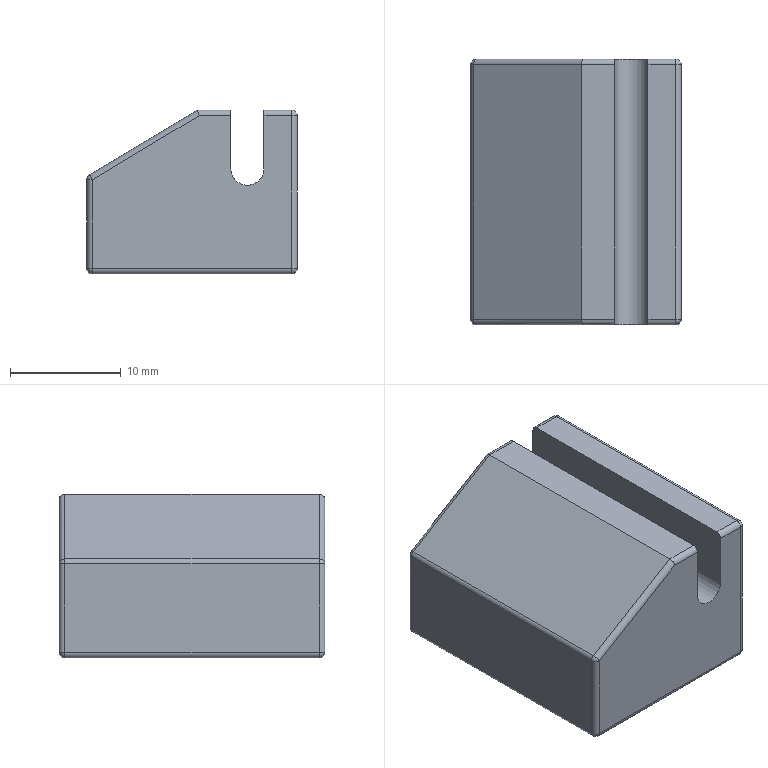Part | STEP file | 2-11.1 | 1 solid | 52 faces | box 19 x 24 x 14.792 mm | volume 4772 mm3 | cylinder 25 | plane 15 | sphere 12 | commonest cylinder face diameters 1 x24 3 x1